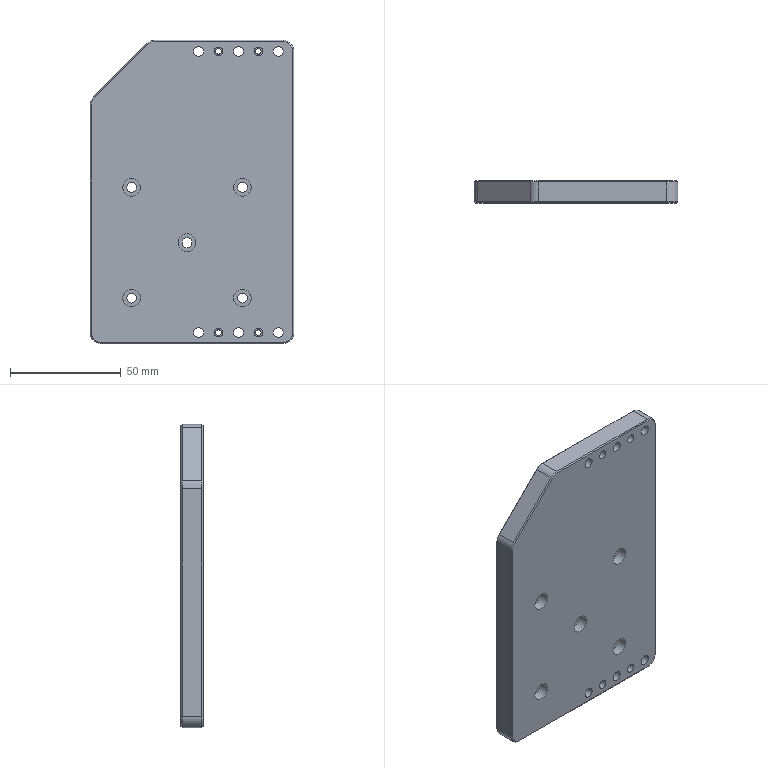Part | 1 solid | 77 faces | box 92 x 10 x 137 mm | volume 118281 mm3 | cylinder 35 | plane 32 | cone 10 | commonest cylinder face diameters 4.5 x11 8 x11 10 x5 2.5 x4 4 x4